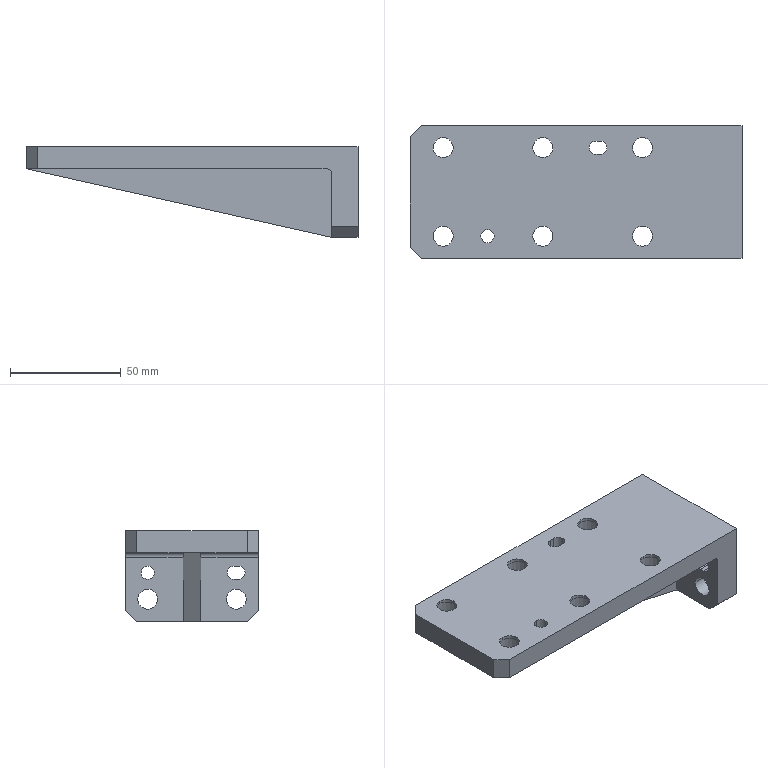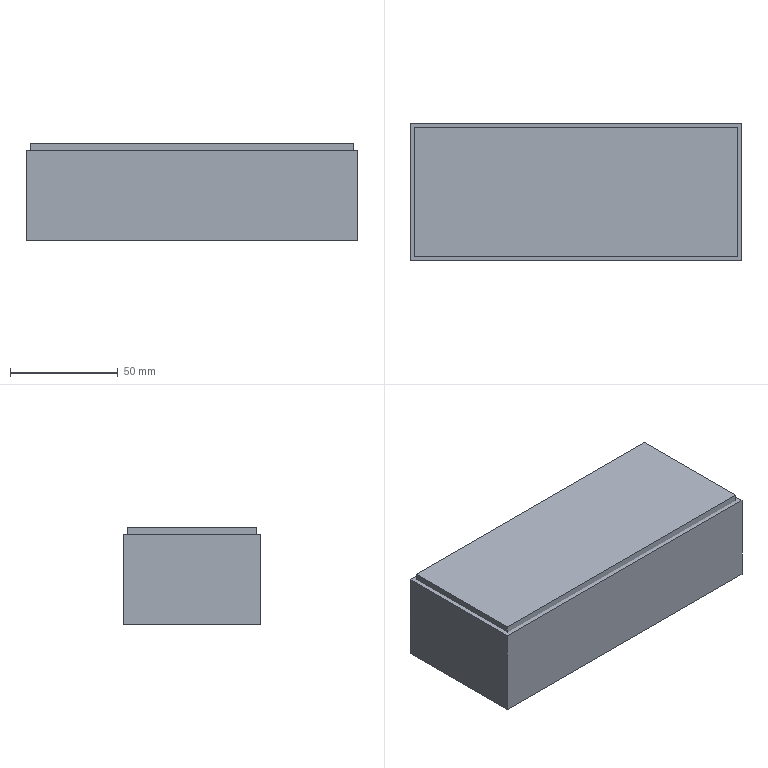CAM job | NX | 3-axis milling, drilling | part box 150 x 60 x 41 mm | stock box 154 x 64 x 45 mm
Tools:
number,name,description,diameter,corner_radius,flute_length,length,flutes
1,D50,Milling Tool-5 Parameters,50.0,0.0,50.0,75.0,2
2,D6A45,Milling Tool-5 Parameters,6.0,0.0,3.0,3.0,2
11,9.0ZT,Drilling Tool,9.0,0.0,35.0,50.0,2
3,D10,Milling Tool-5 Parameters,10.0,0.0,50.0,75.0,2
4,D10JING,Milling Tool-5 Parameters,10.0,0.0,50.0,75.0,2
10,D4,Milling Tool-5 Parameters,4.0,0.0,50.0,75.0,2
20,D6R0.5,Milling Tool-5 Parameters,6.0,0.5,50.0,75.0,2
8,D6,Milling Tool-5 Parameters,6.0,0.0,50.0,75.0,2
Operations:
program,operation,operation_type,tool,method,geometry_group,spindle_rpm,surface_speed,feed_per_tooth,feed_cut,feed_plunge,cut_length_mm,path_length_mm,cut_time_min,machine_time_min
1-153-60-45毛胚-虎钳,FLOOR_WALL,VolumeBased25DMillingOperation,D50,METHOD,A,6500.0,1286.0,0.0962,1250.0,100.0,667.997,721.997,0.5344,0.5398
1-153-60-45毛胚-虎钳,DRILLING_COPY_1,Operation,D6A45,METHOD,A,3000.0,56.0,0.0333,200.0,0.0,40.8,373.74,0.204,0.2373
1-153-60-45毛胚-虎钳,DRILLING_COPY_1_COPY_COPY_COPY_COPY,Operation,9.0ZT,METHOD,A,2000.0,20.0,0.0375,150.0,0.0,100.223,485.983,0.6682,0.7067
1-153-60-45毛胚-虎钳,ADAPTIVE_MILLING,CavityMilling,D10,METHOD,A,7000.0,219.0,0.2143,3000.0,1000.0,2865.883,3133.146,0.9593,0.986
1-153-60-45毛胚-虎钳,ZLEVEL_PROFILE_COPY_COPY_1_COPY_COPY_COPY_1,ZLevelMilling,D10JING,METHOD,A,7000.0,219.0,0.0714,1000.0,100.0,897.381,1039.505,0.8974,0.9116
1-153-60-45毛胚-虎钳,ZLEVEL_PROFILE,ZLevelMilling,D4,METHOD,A,7000.0,87.0,0.1071,1500.0,1000.0,445.928,645.064,0.3151,0.335
1-153-60-45毛胚-虎钳,ZLEVEL_PROFILE_COPY_1_COPY_COPY_COPY_COPY_2_COPY,ZLevelMilling,D6A45,METHOD,A,7000.0,131.0,0.0714,1000.0,1000.0,617.898,1635.765,0.6179,0.7197
1-153-60-45毛胚-虎钳,刀补10,ZLevelMilling,D4,METHOD,A,7000.0,87.0,0.0607,850.0,1000.0,414.435,618.472,0.4871,0.5075
2-153-60-45毛胚-虎钳,FLOOR_WALL_COPY,VolumeBased25DMillingOperation,D50,METHOD,B,6500.0,1286.0,0.0962,1250.0,100.0,1807.988,2131.98,1.446,1.479
2-153-60-45毛胚-虎钳,ADAPTIVE_MILLING_COPY,CavityMilling,D10,METHOD,B,7000.0,219.0,0.2143,3000.0,1000.0,34308.31,51067.099,11.696,13.372
2-153-60-45毛胚-虎钳,ZLEVEL_PROFILE_COPY_COPY_1_COPY_COPY_COPY_1_COPY,ZLevelMilling,D10JING,METHOD,B,7000.0,219.0,0.0714,1000.0,100.0,554.721,1062.073,0.5547,0.6055
2-153-60-45毛胚-虎钳,FLOOR_WALL_1_COPY_1,VolumeBased25DMillingOperation,D10JING,METHOD,B,7000.0,87.0,0.0714,1000.0,100.0,2148.096,2709.531,2.148,2.222
2-153-60-45毛胚-虎钳,HOLE_MILLING,CylinderMilling,D10JING,METHOD,B,7000.0,131.0,0.1071,1500.0,100.0,1214.83,2215.43,0.8099,0.9099
2-153-60-45毛胚-虎钳,ZLEVEL_PROFILE_COPY_COPY_1_COPY_COPY_COPY_1_COPY_COPY_1,ZLevelMilling,D6,METHOD,B,7000.0,131.0,0.1071,1500.0,100.0,773.681,1368.521,0.5158,0.5753
2-153-60-45毛胚-虎钳,ZLEVEL_PROFILE_COPY_COPY_1_COPY_COPY_COPY_1_COPY_COPY,ZLevelMilling,D6R0.5,METHOD,B,7000.0,131.0,0.2143,3000.0,1000.0,21122.124,21213.646,7.041,7.051
2-153-60-45毛胚-虎钳,ZLEVEL_PROFILE_COPY_COPY_1_COPY_COPY_COPY_1_COPY_COPY_COPY,ZLevelMilling,D6R0.5,METHOD,B,7000.0,131.0,0.2143,3000.0,1000.0,1587.711,1870.256,0.5305,0.5588
2-153-60-45毛胚-虎钳,ZLEVEL_PROFILE_COPY_COPY_1_COPY_COPY_COPY_1_COPY_COPY_COPY_1,ZLevelMilling,D6R0.5,METHOD,B,7000.0,131.0,0.2143,3000.0,1000.0,2916.194,3112.495,0.9733,0.9929
2-153-60-45毛胚-虎钳,ZLEVEL_PROFILE_COPY_1_COPY_COPY_COPY_COPY_2_COPY_COPY,ZLevelMilling,D6A45,METHOD,B,7000.0,131.0,0.0714,1000.0,1000.0,122.132,339.77,0.1221,0.1439
2-153-60-45毛胚-虎钳,ZLEVEL_PROFILE_COPY_1_COPY_COPY_COPY_COPY_2_COPY_COPY_COPY,ZLevelMilling,D6A45,METHOD,B,7000.0,131.0,0.0714,1000.0,1000.0,634.12,2156.206,0.6341,0.7863